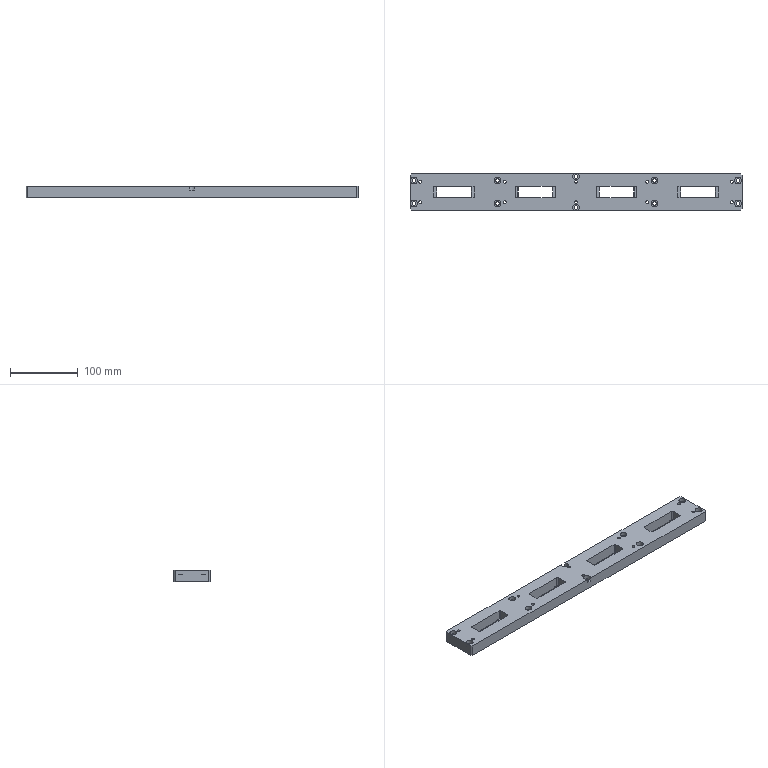NC program | NX | posted with a generic post | part box 490 x 54 x 17 mm
Lines 1 to 1857 of 8955, first 1708 of 1839 lines:
N10 G17 G21 G94 G90
(FLOOR_WALL , TOOL : D80)
N12 T19 M6
N14 G54
N16 G17 G0 G90 X-45. Y-27. S6500 M3
N18 G43 Z30. H19
N20 Z3.
N22 G94 G1 Z0. F1500.
N24 X-42.
N26 X532.
N28 X535.
N30 Z3.
N32 G0 Z30.
N34 M5
(DRILLING , TOOL : D6A45)
N36 T01 M6
N38 G54
N40 G17 G0 G90 X484. Y-10. S5000 M3
N42 G43 Z30. H1
N44 G94 G81 G98 Z-1.8 F350. R3.
N46 X475. Y-12.
N48 X484. Y-44.
N50 X475. Y-42.
N52 X361. Y-44.
N54 X350. Y-42.
N56 X361. Y-10.
N58 X350. Y-12.
N60 X245. Y-4.
N62 Y-12.
N64 Y-42.
N66 Y-50.
N68 X140. Y-42.
N70 X129. Y-44.
N72 X140. Y-12.
N74 X129. Y-10.
N76 X15. Y-12.
N78 X6. Y-10.
N80 X15. Y-42.
N82 X6. Y-44.
N84 G80
N86 G0 X6. Y-44. Z30.
N88 M5
(DRILLING_COPY_COPY , TOOL : 4..2ZT)
N90 T04 M6
N92 G54
N94 G17 G0 G90 X15. Y-12. S2000 M3
N96 G43 Z30. H4
N98 G94 G83 G98 Z-19.762 F300. Q2. R3.
N100 Y-42.
N102 X140.
N104 Y-12.
N106 X245.
N108 Y-42.
N110 X350.
N112 Y-12.
N114 X475.
N116 Y-42.
N118 G80
N120 G0 X475. Y-42. Z30.
N122 M5
(DRILLING_COPY_COPY_COPY , TOOL : 5.5ZT)
N124 T09 M6
N126 G54
N128 G17 G0 G90 X6. Y-10. S2000 M3
N130 G43 Z30. H9
N132 G94 G83 G98 Z-19.152 F300. Q2. R3.
N134 Y-44.
N136 X129.
N138 Y-10.
N140 X245. Y-4.
N142 Y-50.
N144 X361. Y-44.
N146 Y-10.
N148 X484.
N150 Y-44.
N152 G80
N154 G0 X484. Y-44. Z30.
N156 M5
(ZLEVEL_PROFILE , TOOL : D10)
N158 T15 M6
N160 G54
N162 G17 G0 G90 X423.853 Y-23.5 S8500 M3
N164 G43 Z30. H15
N166 Z1.5
N168 G94 G1 X400.1 Z0.255 F1000.
N170 Y-30.5 Z-0.112
N172 X425. Z-1.417
N174 X449.9 F3000.
N176 Y-23.5
N178 X400.1
N180 Y-30.5
N182 X425.
N184 X449.9 Z-1.727
N186 Y-23.5 Z-1.814
N188 X410.06 Z-2.311
N190 X405.08 Z-2.373
N192 X400.1 Z-2.436
N194 Y-30.5 Z-2.523
N196 X425. Z-2.833
N198 X449.9 Z-3.144
N200 Y-23.5 Z-3.231
N202 X410.06 Z-3.728
N204 X405.08 Z-3.79
N206 X400.1 Z-3.852
N208 Y-30.5 Z-3.939
N210 X425. Z-4.25
N212 X449.9 Z-4.561
N214 Y-23.5 Z-4.648
N216 X410.06 Z-5.145
N218 X405.08 Z-5.207
N220 X400.1 Z-5.269
N222 Y-30.5 Z-5.356
N224 X425. Z-5.667
N226 X449.9 Z-5.977
N228 Y-23.5 Z-6.064
N230 X410.06 Z-6.561
N232 X405.08 Z-6.623
N234 X400.1 Z-6.686
N236 Y-30.5 Z-6.773
N238 X425. Z-7.083
N240 X449.9 Z-7.394
N242 Y-23.5 Z-7.481
N244 X410.06 Z-7.978
N246 X405.08 Z-8.04
N248 X400.1 Y-23.501 Z-8.102
N250 Y-30.5 Z-8.189
N252 X425. Z-8.5
N254 X449.9 Z-8.811
N256 Y-23.5 Z-8.898
N258 X410.061 Z-9.395
N260 X405.08 Z-9.457
N262 X400.1 Y-23.501 Z-9.519
N264 Y-30.5 Z-9.606
N266 X425. Z-9.917
N268 X449.9 Z-10.227
N270 Y-23.5 Z-10.314
N272 X410.061 Z-10.811
N274 X405.08 Z-10.873
N276 X400.1 Y-23.501 Z-10.936
N278 Y-30.5 Z-11.023
N280 X425. Z-11.333
N282 X449.9 Z-11.644
N284 Y-23.5 Z-11.731
N286 X410.061 Z-12.228
N288 X405.08 Z-12.29
N290 X400.1 Y-23.501 Z-12.352
N292 Y-30.5 Z-12.439
N294 X425. Z-12.75
N296 X449.9 Z-13.061
N298 Y-23.5 Z-13.148
N300 X410.061 Z-13.645
N302 X405.08 Z-13.707
N304 X400.1 Y-23.501 Z-13.769
N306 Y-30.5 Z-13.856
N308 X425. Z-14.167
N310 X441.6 Z-14.391
N312 X443.734 Z-14.441
N314 X445.868 Z-14.491
N316 X445.866 Y-30.366 Z-14.492
N318 X445.773 Y-23.503 Z-14.585
N320 X442.858 Y-23.5 Z-14.644
N322 X439.94 Z-14.703
N324 X410.061 Z-15.108
N326 X407.33 Z-15.153
N328 X404.6 Y-23.501 Z-15.199
N330 Y-30.345 Z-15.292
N332 Y-30.5
N334 X408.4 Z-15.294
N336 X416.7 Z-15.359
N338 X425. Z-15.471
N340 Z-15.583
N342 X438.602 Z-15.785
N344 X442.003 Z-15.835
N346 X445.4 Y-30.497 Z-15.886
N348 Y-30.369 Z-15.888
N350 Y-23.5 Z-15.989
N352 X404.6 Z-16.594
N354 Y-30.497 Z-16.698
N356 X407.998 Y-30.5 Z-16.748
N358 X411.399 Z-16.798
N360 X425. Z-17.
N362 X445.403
N364 X445.4 Y-30.366
N366 Y-23.5
N368 X404.6
N370 Y-30.5
N372 X425.
N374 Z-15.5
N376 G0 Z30.
N378 X303.853 Y-23.5
N380 Z1.5
N382 G1 X280.1 Z0.255 F1000.
N384 Y-30.5 Z-0.112
N386 X305. Z-1.417
N388 X329.9 F3000.
N390 Y-23.5
N392 X280.1
N394 Y-30.5
N396 X305.
N398 X329.9 Z-1.727
N400 Y-23.5 Z-1.814
N402 X290.06 Z-2.311
N404 X285.08 Z-2.373
N406 X280.1 Z-2.436
N408 Y-30.5 Z-2.523
N410 X305. Z-2.833
N412 X329.9 Z-3.144
N414 Y-23.5 Z-3.231
N416 X290.06 Z-3.728
N418 X285.08 Z-3.79
N420 X280.1 Z-3.852
N422 Y-30.5 Z-3.939
N424 X305. Z-4.25
N426 X329.9 Z-4.561
N428 Y-23.5 Z-4.648
N430 X290.06 Z-5.145
N432 X285.08 Z-5.207
N434 X280.1 Z-5.269
N436 Y-30.5 Z-5.356
N438 X305. Z-5.667
N440 X329.9 Z-5.977
N442 Y-23.5 Z-6.064
N444 X290.06 Z-6.561
N446 X285.08 Z-6.623
N448 X280.1 Z-6.686
N450 Y-30.5 Z-6.773
N452 X305. Z-7.083
N454 X329.9 Z-7.394
N456 Y-23.5 Z-7.481
N458 X290.06 Z-7.978
N460 X285.08 Z-8.04
N462 X280.1 Y-23.501 Z-8.102
N464 Y-30.5 Z-8.189
N466 X305. Z-8.5
N468 X329.9 Z-8.811
N470 Y-23.5 Z-8.898
N472 X290.061 Z-9.395
N474 X285.08 Z-9.457
N476 X280.1 Y-23.501 Z-9.519
N478 Y-30.5 Z-9.606
N480 X305. Z-9.917
N482 X329.9 Z-10.227
N484 Y-23.5 Z-10.314
N486 X290.061 Z-10.811
N488 X285.08 Z-10.873
N490 X280.1 Y-23.501 Z-10.936
N492 Y-30.5 Z-11.023
N494 X305. Z-11.333
N496 X329.9 Z-11.644
N498 Y-23.5 Z-11.731
N500 X290.061 Z-12.228
N502 X285.08 Z-12.29
N504 X280.1 Y-23.501 Z-12.352
N506 Y-30.5 Z-12.439
N508 X305. Z-12.75
N510 X329.9 Z-13.061
N512 Y-23.5 Z-13.148
N514 X290.061 Z-13.645
N516 X285.08 Z-13.707
N518 X280.1 Y-23.501 Z-13.769
N520 Y-30.5 Z-13.856
N522 X305. Z-14.167
N524 X321.6 Z-14.391
N526 X323.734 Z-14.441
N528 X325.868 Z-14.491
N530 X325.867 Y-30.389 Z-14.492
N532 X325.773 Y-23.503 Z-14.585
N534 X322.858 Y-23.5 Z-14.644
N536 X319.94 Z-14.703
N538 X290.061 Z-15.108
N540 X287.33 Z-15.153
N542 X284.6 Y-23.501 Z-15.199
N544 Y-30.497 Z-15.294
N546 X286.499 Y-30.5 Z-15.326
N548 X288.4 Z-15.359
N550 X305. Z-15.583
N552 X318.602 Z-15.785
N554 X322.002 Z-15.835
N556 X325.4 Y-30.497 Z-15.886
N558 Y-30.389 Z-15.887
N560 Y-23.5 Z-15.989
N562 X284.6 Z-16.594
N564 Y-30.5 Z-16.698
N566 X305. Z-17.
N568 X325.402
N570 X325.4 Y-30.389
N572 Y-23.5
N574 X284.6
N576 Y-30.5
N578 X305.
N580 Z-15.5
N582 G0 Z30.
N584 X183.853 Y-23.5
N586 Z1.5
N588 G1 X160.1 Z0.255 F1000.
N590 Y-30.5 Z-0.112
N592 X185. Z-1.417
N594 X209.9 F3000.
N596 Y-23.5
N598 X160.1
N600 Y-30.5
N602 X185.
N604 X209.9 Z-1.727
N606 Y-23.5 Z-1.814
N608 X160.1 Z-2.436
N610 Y-30.5 Z-2.523
N612 X185. Z-2.833
N614 X209.9 Z-3.144
N616 Y-23.5 Z-3.231
N618 X160.1 Z-3.852
N620 Y-30.5 Z-3.939
N622 X185. Z-4.25
N624 X209.9 Z-4.561
N626 Y-23.5 Z-4.648
N628 X160.1 Z-5.269
N630 Y-30.5 Z-5.356
N632 X185. Z-5.667
N634 X209.9 Z-5.977
N636 Y-23.5 Z-6.064
N638 X160.1 Z-6.686
N640 Y-30.5 Z-6.773
N642 X185. Z-7.083
N644 X209.9 Z-7.394
N646 Y-23.5 Z-7.481
N648 X160.1 Z-8.102
N650 Y-30.5 Z-8.189
N652 X185. Z-8.5
N654 X209.9 Z-8.811
N656 Y-23.5 Z-8.898
N658 X160.1 Z-9.519
N660 Y-30.5 Z-9.606
N662 X185. Z-9.917
N664 X209.9 Z-10.227
N666 Y-23.5 Z-10.314
N668 X160.1 Z-10.936
N670 Y-30.5 Z-11.023
N672 X185. Z-11.333
N674 X209.9 Z-11.644
N676 Y-23.5 Z-11.731
N678 X160.1 Z-12.352
N680 Y-30.5 Z-12.439
N682 X185. Z-12.75
N684 X209.9 Z-13.061
N686 Y-23.5 Z-13.148
N688 X160.1 Z-13.769
N690 Y-30.5 Z-13.856
N692 X185. Z-14.167
N694 X201.6 Z-14.391
N696 X203.736 Z-14.441
N698 X205.868 Y-30.497 Z-14.491
N700 X205.773 Y-23.503 Z-14.585
N702 X202.858 Y-23.5 Z-14.644
N704 X199.94 Z-14.703
N706 X170.06 Z-15.108
N708 X167.329 Z-15.153
N710 X164.6 Y-23.503 Z-15.199
N712 Y-30.497 Z-15.294
N714 X166.499 Y-30.5 Z-15.326
N716 X168.4 Z-15.359
N718 X185. Z-15.583
N720 X205.4 Z-15.886
N722 Y-23.5 Z-15.989
N724 X164.6 Z-16.594
N726 Y-30.5 Z-16.698
N728 X185. Z-17.
N730 X205.4
N732 Y-23.5
N734 X164.6
N736 Y-30.5
N738 X185.
N740 Z-15.5
N742 G0 Z30.
N744 X63.853 Y-23.5
N746 Z1.5
N748 G1 X40.1 Z0.255 F1000.
N750 Y-30.5 Z-0.112
N752 X65. Z-1.417
N754 X89.9 F3000.
N756 Y-23.5
N758 X40.1
N760 Y-30.5
N762 X65.
N764 X89.9 Z-1.727
N766 Y-23.5 Z-1.814
N768 X84.92 Z-1.877
N770 X79.94 Z-1.939
N772 X50.06 Z-2.311
N774 X45.08 Z-2.373
N776 X40.1 Z-2.436
N778 Y-30.5 Z-2.523
N780 X65. Z-2.833
N782 X89.9 Z-3.144
N784 Y-23.5 Z-3.231
N786 X84.92 Z-3.293
N788 X79.94 Z-3.355
N790 X50.06 Z-3.728
N792 X45.08 Z-3.79
N794 X40.1 Z-3.852
N796 Y-30.5 Z-3.939
N798 X65. Z-4.25
N800 X89.9 Z-4.561
N802 Y-23.5 Z-4.648
N804 X84.92 Z-4.71
N806 X79.94 Z-4.772
N808 X50.06 Z-5.145
N810 X45.08 Z-5.207
N812 X40.1 Z-5.269
N814 Y-30.5 Z-5.356
N816 X65. Z-5.667
N818 X89.9 Z-5.977
N820 Y-23.5 Z-6.064
N822 X84.92 Z-6.127
N824 X79.94 Z-6.189
N826 X50.06 Z-6.561
N828 X45.08 Z-6.623
N830 X40.1 Z-6.686
N832 Y-30.5 Z-6.773
N834 X65. Z-7.083
N836 X89.9 Z-7.394
N838 Y-23.5 Z-7.481
N840 X84.92 Z-7.543
N842 X79.94 Z-7.605
N844 X50.06 Z-7.978
N846 X45.08 Z-8.04
N848 X40.1 Y-23.501 Z-8.102
N850 Y-30.5 Z-8.189
N852 X65. Z-8.5
N854 X89.9 Z-8.811
N856 Y-23.5 Z-8.898
N858 X84.92 Z-8.96
N860 X79.94 Z-9.022
N862 X50.061 Z-9.395
N864 X45.08 Z-9.457
N866 X40.1 Y-23.501 Z-9.519
N868 Y-30.5 Z-9.606
N870 X65. Z-9.917
N872 X89.9 Z-10.227
N874 Y-23.5 Z-10.314
N876 X84.92 Z-10.377
N878 X79.94 Z-10.439
N880 X50.061 Z-10.811
N882 X45.08 Z-10.873
N884 X40.1 Y-23.501 Z-10.936
N886 Y-30.5 Z-11.023
N888 X65. Z-11.333
N890 X89.9 Z-11.644
N892 Y-23.5 Z-11.731
N894 X84.92 Z-11.793
N896 X79.94 Z-11.855
N898 X50.061 Z-12.228
N900 X45.08 Z-12.29
N902 X40.1 Y-23.501 Z-12.352
N904 Y-30.5 Z-12.439
N906 X65. Z-12.75
N908 X89.9 Z-13.061
N910 Y-23.5 Z-13.148
N912 X84.92 Z-13.21
N914 X79.94 Z-13.272
N916 X50.061 Z-13.645
N918 X45.08 Z-13.707
N920 X40.1 Y-23.501 Z-13.769
N922 Y-30.5 Z-13.856
N924 X65. Z-14.167
N926 X81.6 Z-14.391
N928 X83.734 Z-14.441
N930 X85.868 Z-14.491
N932 X85.866 Y-30.345 Z-14.493
N934 X85.773 Y-23.503 Z-14.585
N936 X82.858 Y-23.5 Z-14.644
N938 X79.94 Z-14.703
N940 X50.061 Z-15.108
N942 X47.33 Z-15.153
N944 X44.6 Y-23.501 Z-15.199
N946 Y-30.366 Z-15.292
N948 Y-30.5
N950 X48.4 Z-15.294
N952 X56.7 Z-15.359
N954 X65. Z-15.471
N956 Z-15.583
N958 X78.602 Z-15.785
N960 X82.002 Z-15.835
N962 X85.4 Y-30.497 Z-15.886
N964 Y-30.348 Z-15.888
N966 Y-23.5 Z-15.989
N968 X44.6 Z-16.594
N970 Y-26.934 Z-16.645
N972 Y-30.497 Z-16.698
N974 X47.997 Y-30.5 Z-16.748
N976 X51.398 Z-16.798
N978 X65. Z-17.
N980 X85.402
N982 X85.4 Y-30.345
N984 Y-23.5
N986 X44.6
N988 Y-30.366
N990 X44.597 Y-30.5
N992 X65.
N994 Z-15.5
N996 G0 Z30.
N998 X66.446 Y5.1
N1000 Z1.5
N1002 G1 X122.099 Z-1.417 F1000.
N1004 X242.198 F3000.
N1006 Y5.096
N1008 G2 X245. Y4.124 R5.1
N1010 X247.817 Y5.097 R5.1
N1012 G1 Y5.1
N1014 X488.
N1016 G2 X491.606 Y3.606 R5.1
N1018 G1 X493.606 Y1.606
N1020 G2 X495.1 Y-2. R5.1
N1022 G1 Y-52.
N1024 G2 X493.606 Y-55.606 R5.1
N1026 G1 X491.606 Y-57.606
N1028 G2 X488. Y-59.1 R5.1
N1030 G1 X248.
N1032 G2 X245. Y-58.124 R5.1
N1034 X242. Y-59.1 R5.1
N1036 G1 X2.
N1038 G2 X-1.606 Y-57.606 R5.1
N1040 G1 X-3.606 Y-55.606
N1042 G2 X-5.1 Y-52. R5.1
N1044 G1 Y-2.
N1046 G2 X-3.606 Y1.606 R5.1
N1048 G1 X-1.606 Y3.606
N1050 G2 X2. Y5.1 R5.1
N1052 G1 X122.099
N1054 X232.96 Z-1.557
N1056 X237.58 Z-1.563
N1058 X242.198 Y5.096 Z-1.569
N1060 X242.708 Y5.051 Z-1.57
N1062 X243.19 Y4.959
N1064 X243.671 Y4.818 Z-1.571
N1066 X244.136 Y4.631 Z-1.572
N1068 X244.574 Y4.403
N1070 X245. Y4.124 Z-1.573
N1072 X245.429 Y4.404 Z-1.574
N1074 X245.868 Y4.633
N1076 X246.336 Y4.821 Z-1.575
N1078 X246.82 Y4.962
N1080 X247.305 Y5.052 Z-1.576
N1082 X247.817 Y5.097 Z-1.577
N1084 X252.62 Y5.1 Z-1.583
N1086 X257.425 Z-1.589
N1088 X488. Z-1.882
N1090 X488.5 Y5.075
N1092 X488.995 Y5.002 Z-1.883
N1094 X489.48 Y4.88 Z-1.884
N1096 X489.952 Y4.712
N1098 X490.404 Y4.498 Z-1.885
N1100 X490.833 Y4.24
N1102 X491.235 Y3.942 Z-1.886
N1104 X491.606 Y3.606 Z-1.887
N1106 X493.606 Y1.606 Z-1.89
N1108 X493.942 Y1.235 Z-1.891
N1110 X494.24 Y0.833 Z-1.892
N1112 X494.498 Y0.404
N1114 X494.712 Y-0.048 Z-1.893
N1116 X494.88 Y-0.52
N1118 X495.002 Y-1.005 Z-1.894
N1120 X495.075 Y-1.5 Z-1.895
N1122 X495.1 Y-2.
N1124 Y-52. Z-1.959
N1126 X495.075 Y-52.5
N1128 X495.002 Y-52.995 Z-1.96
N1130 X494.88 Y-53.48 Z-1.961
N1132 X494.712 Y-53.952
N1134 X494.498 Y-54.404 Z-1.962
N1136 X494.24 Y-54.833 Z-1.963
N1138 X493.942 Y-55.235
N1140 X493.606 Y-55.606 Z-1.964
N1142 X491.606 Y-57.606 Z-1.967
N1144 X491.235 Y-57.942 Z-1.968
N1146 X490.833 Y-58.24 Z-1.969
N1148 X490.404 Y-58.498
N1150 X489.952 Y-58.712 Z-1.97
N1152 X489.48 Y-58.88 Z-1.971
N1154 X488.995 Y-59.002
N1156 X488.5 Y-59.075 Z-1.972
N1158 X488. Y-59.1 Z-1.973
N1160 X248. Z-2.277
N1162 X247.466 Y-59.072 Z-2.278
N1164 X246.939 Y-58.988 Z-2.279
N1166 X246.423 Y-58.85
N1168 X245.924 Y-58.658 Z-2.28
N1170 X245.456 Y-58.42 Z-2.281
N1172 X245. Y-58.124
N1174 X244.544 Y-58.42 Z-2.282
N1176 X244.076 Y-58.658 Z-2.283
N1178 X243.577 Y-58.85
N1180 X243.061 Y-58.988 Z-2.284
N1182 X242.534 Y-59.072 Z-2.285
N1184 X242. Y-59.1
N1186 X2. Z-2.59
N1188 X1.5 Y-59.075 Z-2.591
N1190 X1.005 Y-59.002
N1192 X0.52 Y-58.88 Z-2.592
N1194 X0.048 Y-58.712
N1196 X-0.404 Y-58.498 Z-2.593
N1198 X-0.833 Y-58.24 Z-2.594
N1200 X-1.235 Y-57.942
N1202 X-1.606 Y-57.606 Z-2.595
N1204 X-3.606 Y-55.606 Z-2.599
N1206 X-3.942 Y-55.235
N1208 X-4.24 Y-54.833 Z-2.6
N1210 X-4.498 Y-54.404 Z-2.601
N1212 X-4.712 Y-53.952
N1214 X-4.88 Y-53.48 Z-2.602
N1216 X-5.002 Y-52.995
N1218 X-5.075 Y-52.5 Z-2.603
N1220 X-5.1 Y-52. Z-2.604
N1222 Y-2. Z-2.667
N1224 X-5.075 Y-1.5 Z-2.668
N1226 X-5.002 Y-1.005
N1228 X-4.88 Y-0.52 Z-2.669
N1230 X-4.712 Y-0.048 Z-2.67
N1232 X-4.498 Y0.404
N1234 X-4.24 Y0.833 Z-2.671
N1236 X-3.942 Y1.235 Z-2.672
N1238 X-3.606 Y1.606
N1240 X-1.606 Y3.606 Z-2.676
N1242 X-1.235 Y3.942
N1244 X-0.833 Y4.24 Z-2.677
N1246 X-0.404 Y4.498 Z-2.678
N1248 X0.048 Y4.712
N1250 X0.52 Y4.88 Z-2.679
N1252 X1.005 Y5.002 Z-2.68
N1254 X1.5 Y5.075
N1256 X2. Y5.1 Z-2.681
N1258 X122.099 Z-2.833
N1260 X232.96 Z-2.974
N1262 X237.58 Z-2.98
N1264 X242.198 Y5.096 Z-2.986
N1266 X242.708 Y5.051
N1268 X243.19 Y4.959 Z-2.987
N1270 X243.671 Y4.818 Z-2.988
N1272 X244.136 Y4.631
N1274 X244.574 Y4.403 Z-2.989
N1276 X245. Y4.124 Z-2.99
N1278 X245.429 Y4.404
N1280 X245.868 Y4.633 Z-2.991
N1282 X246.336 Y4.821 Z-2.992
N1284 X246.82 Y4.962
N1286 X247.305 Y5.052 Z-2.993
N1288 X247.817 Y5.097
N1290 X252.62 Y5.1 Z-3.
N1292 X257.425 Z-3.006
N1294 X488. Z-3.298
N1296 X488.5 Y5.075 Z-3.299
N1298 X488.995 Y5.002 Z-3.3
N1300 X489.48 Y4.88
N1302 X489.952 Y4.712 Z-3.301
N1304 X490.404 Y4.498
N1306 X490.833 Y4.24 Z-3.302
N1308 X491.235 Y3.942 Z-3.303
N1310 X491.606 Y3.606
N1312 X493.606 Y1.606 Z-3.307
N1314 X493.942 Y1.235 Z-3.308
N1316 X494.24 Y0.833
N1318 X494.498 Y0.404 Z-3.309
N1320 X494.712 Y-0.048
N1322 X494.88 Y-0.52 Z-3.31
N1324 X495.002 Y-1.005 Z-3.311
N1326 X495.075 Y-1.5
N1328 X495.1 Y-2. Z-3.312
N1330 Y-52. Z-3.375
N1332 X495.075 Y-52.5 Z-3.376
N1334 X495.002 Y-52.995 Z-3.377
N1336 X494.88 Y-53.48
N1338 X494.712 Y-53.952 Z-3.378
N1340 X494.498 Y-54.404 Z-3.379
N1342 X494.24 Y-54.833
N1344 X493.942 Y-55.235 Z-3.38
N1346 X493.606 Y-55.606 Z-3.381
N1348 X491.606 Y-57.606 Z-3.384
N1350 X491.235 Y-57.942 Z-3.385
N1352 X490.833 Y-58.24
N1354 X490.404 Y-58.498 Z-3.386
N1356 X489.952 Y-58.712 Z-3.387
N1358 X489.48 Y-58.88
N1360 X488.995 Y-59.002 Z-3.388
N1362 X488.5 Y-59.075 Z-3.389
N1364 X488. Y-59.1
N1366 X248. Z-3.694
N1368 X247.466 Y-59.072 Z-3.695
N1370 X246.939 Y-58.988
N1372 X246.423 Y-58.85 Z-3.696
N1374 X245.924 Y-58.658 Z-3.697
N1376 X245.456 Y-58.42
N1378 X245. Y-58.124 Z-3.698
N1380 X244.544 Y-58.42 Z-3.699
N1382 X244.076 Y-58.658
N1384 X243.577 Y-58.85 Z-3.7
N1386 X243.061 Y-58.988 Z-3.701
N1388 X242.534 Y-59.072
N1390 X242. Y-59.1 Z-3.702
N1392 X2. Z-4.007
N1394 X1.5 Y-59.075
N1396 X1.005 Y-59.002 Z-4.008
N1398 X0.52 Y-58.88 Z-4.009
N1400 X0.048 Y-58.712
N1402 X-0.404 Y-58.498 Z-4.01
N1404 X-0.833 Y-58.24
N1406 X-1.235 Y-57.942 Z-4.011
N1408 X-1.606 Y-57.606 Z-4.012
N1410 X-3.606 Y-55.606 Z-4.015
N1412 X-3.942 Y-55.235 Z-4.016
N1414 X-4.24 Y-54.833 Z-4.017
N1416 X-4.498 Y-54.404
N1418 X-4.712 Y-53.952 Z-4.018
N1420 X-4.88 Y-53.48
N1422 X-5.002 Y-52.995 Z-4.019
N1424 X-5.075 Y-52.5 Z-4.02
N1426 X-5.1 Y-52.
N1428 Y-2. Z-4.084
N1430 X-5.075 Y-1.5
N1432 X-5.002 Y-1.005 Z-4.085
N1434 X-4.88 Y-0.52 Z-4.086
N1436 X-4.712 Y-0.048
N1438 X-4.498 Y0.404 Z-4.087
N1440 X-4.24 Y0.833 Z-4.088
N1442 X-3.942 Y1.235
N1444 X-3.606 Y1.606 Z-4.089
N1446 X-1.606 Y3.606 Z-4.092
N1448 X-1.235 Y3.942 Z-4.093
N1450 X-0.833 Y4.24 Z-4.094
N1452 X-0.404 Y4.498
N1454 X0.048 Y4.712 Z-4.095
N1456 X0.52 Y4.88 Z-4.096
N1458 X1.005 Y5.002
N1460 X1.5 Y5.075 Z-4.097
N1462 X2. Y5.1 Z-4.098
N1464 X122.099 Z-4.25
N1466 X232.96 Z-4.391
N1468 X237.578 Z-4.397
N1470 X242.194 Y5.096 Z-4.402
N1472 X242.34 Y5.089 Z-4.403
N1474 X242.766 Y5.042
N1476 X243.19 Y4.959 Z-4.404
N1478 X243.663 Y4.821
N1480 X244.136 Y4.631 Z-4.405
N1482 X244.568 Y4.406 Z-4.406
N1484 X245. Y4.124
N1486 X245.434 Y4.408 Z-4.407
N1488 X245.868 Y4.633 Z-4.408
N1490 X246.344 Y4.824
N1492 X246.82 Y4.962 Z-4.409
N1494 X247.239 Y5.043
N1496 X247.66 Y5.089 Z-4.41
N1498 X247.821 Y5.097
N1500 X252.622 Y5.1 Z-4.416
N1502 X257.425 Z-4.422
N1504 X488. Z-4.715
N1506 X488.5 Y5.075 Z-4.716
N1508 X488.995 Y5.002
N1510 X489.48 Y4.88 Z-4.717
N1512 X489.952 Y4.712 Z-4.718
N1514 X490.404 Y4.498
N1516 X490.833 Y4.24 Z-4.719
N1518 X491.235 Y3.942
N1520 X491.606 Y3.606 Z-4.72
N1522 X493.606 Y1.606 Z-4.724
N1524 X493.942 Y1.235
N1526 X494.24 Y0.833 Z-4.725
N1528 X494.498 Y0.404 Z-4.726
N1530 X494.712 Y-0.048
N1532 X494.88 Y-0.52 Z-4.727
N1534 X495.002 Y-1.005 Z-4.728
N1536 X495.075 Y-1.5
N1538 X495.1 Y-2. Z-4.729
N1540 Y-52. Z-4.792
N1542 X495.075 Y-52.5 Z-4.793
N1544 X495.002 Y-52.995 Z-4.794
N1546 X494.88 Y-53.48
N1548 X494.712 Y-53.952 Z-4.795
N1550 X494.498 Y-54.404
N1552 X494.24 Y-54.833 Z-4.796
N1554 X493.942 Y-55.235 Z-4.797
N1556 X493.606 Y-55.606
N1558 X491.606 Y-57.606 Z-4.801
N1560 X491.235 Y-57.942 Z-4.802
N1562 X490.833 Y-58.24
N1564 X490.404 Y-58.498 Z-4.803
N1566 X489.952 Y-58.712
N1568 X489.48 Y-58.88 Z-4.804
N1570 X488.995 Y-59.002 Z-4.805
N1572 X488.5 Y-59.075
N1574 X488. Y-59.1 Z-4.806
N1576 X248. Z-5.111
N1578 X247.469 Y-59.072
N1580 X246.939 Y-58.988 Z-5.112
N1582 X246.431 Y-58.853 Z-5.113
N1584 X245.924 Y-58.658
N1586 X245.462 Y-58.424 Z-5.114
N1588 X245. Y-58.124 Z-5.115
N1590 X244.538 Y-58.424
N1592 X244.076 Y-58.658 Z-5.116
N1594 X243.569 Y-58.853
N1596 X243.061 Y-58.988 Z-5.117
N1598 X242.531 Y-59.072 Z-5.118
N1600 X242. Y-59.1
N1602 X2. Z-5.423
N1604 X1.5 Y-59.075 Z-5.424
N1606 X1.005 Y-59.002
N1608 X0.52 Y-58.88 Z-5.425
N1610 X0.048 Y-58.712 Z-5.426
N1612 X-0.404 Y-58.498
N1614 X-0.833 Y-58.24 Z-5.427
N1616 X-1.235 Y-57.942 Z-5.428
N1618 X-1.606 Y-57.606
N1620 X-3.606 Y-55.606 Z-5.432
N1622 X-3.942 Y-55.235
N1624 X-4.24 Y-54.833 Z-5.433
N1626 X-4.498 Y-54.404 Z-5.434
N1628 X-4.712 Y-53.952
N1630 X-4.88 Y-53.48 Z-5.435
N1632 X-5.002 Y-52.995 Z-5.436
N1634 X-5.075 Y-52.5
N1636 X-5.1 Y-52. Z-5.437
N1638 Y-2. Z-5.5
N1640 X-5.075 Y-1.5 Z-5.501
N1642 X-5.002 Y-1.005 Z-5.502
N1644 X-4.88 Y-0.52
N1646 X-4.712 Y-0.048 Z-5.503
N1648 X-4.498 Y0.404 Z-5.504
N1650 X-4.24 Y0.833
N1652 X-3.942 Y1.235 Z-5.505
N1654 X-3.606 Y1.606 Z-5.506
N1656 X-1.606 Y3.606 Z-5.509
N1658 X-1.235 Y3.942 Z-5.51
N1660 X-0.833 Y4.24
N1662 X-0.404 Y4.498 Z-5.511
N1664 X0.048 Y4.712 Z-5.512
N1666 X0.52 Y4.88
N1668 X1.005 Y5.002 Z-5.513
N1670 X1.5 Y5.075 Z-5.514
N1672 X2. Y5.1
N1674 X122.099 Z-5.667
N1676 X242.34 Z-5.819
N1678 X257.425 Z-5.839
N1680 X488. Z-6.131
N1682 X488.5 Y5.075 Z-6.132
N1684 X488.995 Y5.002 Z-6.133
N1686 X489.48 Y4.88
N1688 X489.952 Y4.712 Z-6.134
N1690 X490.404 Y4.498 Z-6.135
N1692 X490.833 Y4.24
N1694 X491.235 Y3.942 Z-6.136
N1696 X491.606 Y3.606 Z-6.137
N1698 X493.606 Y1.606 Z-6.14
N1700 X493.942 Y1.235 Z-6.141
N1702 X494.24 Y0.833
N1704 X494.498 Y0.404 Z-6.142
N1706 X494.712 Y-0.048 Z-6.143
N1708 X494.88 Y-0.52
N1710 X495.002 Y-1.005 Z-6.144
N1712 X495.075 Y-1.5 Z-6.145
N1714 X495.1 Y-2.
N1716 Y-52. Z-6.209
N1718 X495.075 Y-52.5
N1720 X495.002 Y-52.995 Z-6.21
N1722 X494.88 Y-53.48 Z-6.211
N1724 X494.712 Y-53.952
N1726 X494.498 Y-54.404 Z-6.212
N1728 X494.24 Y-54.833 Z-6.213
N1730 X493.942 Y-55.235
N1732 X493.606 Y-55.606 Z-6.214
N1734 X491.606 Y-57.606 Z-6.217
N1736 X491.235 Y-57.942 Z-6.218
N1738 X490.833 Y-58.24 Z-6.219
N1740 X490.404 Y-58.498
N1742 X489.952 Y-58.712 Z-6.22
N1744 X489.48 Y-58.88 Z-6.221
N1746 X488.995 Y-59.002
N1748 X488.5 Y-59.075 Z-6.222
N1750 X488. Y-59.1
N1752 X247.878 Z-6.527
N1754 X232. Z-6.548
N1756 X2. Z-6.84
N1758 X1.5 Y-59.075
N1760 X1.005 Y-59.002 Z-6.841
N1762 X0.52 Y-58.88 Z-6.842
N1764 X0.048 Y-58.712
N1766 X-0.404 Y-58.498 Z-6.843
N1768 X-0.833 Y-58.24 Z-6.844
N1770 X-1.235 Y-57.942
N1772 X-1.606 Y-57.606 Z-6.845
N1774 X-3.606 Y-55.606 Z-6.848
N1776 X-3.942 Y-55.235 Z-6.849
N1778 X-4.24 Y-54.833 Z-6.85
N1780 X-4.498 Y-54.404
N1782 X-4.712 Y-53.952 Z-6.851
N1784 X-4.88 Y-53.48 Z-6.852
N1786 X-5.002 Y-52.995
N1788 X-5.075 Y-52.5 Z-6.853
N1790 X-5.1 Y-52. Z-6.854
N1792 Y-2. Z-6.917
N1794 X-5.075 Y-1.5 Z-6.918
N1796 X-5.002 Y-1.005
N1798 X-4.88 Y-0.52 Z-6.919
N1800 X-4.712 Y-0.048 Z-6.92
N1802 X-4.498 Y0.404
N1804 X-4.24 Y0.833 Z-6.921
N1806 X-3.942 Y1.235
N1808 X-3.606 Y1.606 Z-6.922
N1810 X-1.606 Y3.606 Z-6.926
N1812 X-1.235 Y3.942
N1814 X-0.833 Y4.24 Z-6.927
N1816 X-0.404 Y4.498 Z-6.928
N1818 X0.048 Y4.712
N1820 X0.52 Y4.88 Z-6.929
N1822 X1.005 Y5.002 Z-6.93
N1824 X1.5 Y5.075
N1826 X2. Y5.1 Z-6.931
N1828 X122.099 Z-7.083
N1830 X488. Z-7.548
N1832 X488.5 Y5.075 Z-7.549
N1834 X488.995 Y5.002
N1836 X489.48 Y4.88 Z-7.55
N1838 X489.952 Y4.712 Z-7.551
N1840 X490.404 Y4.498
N1842 X490.833 Y4.24 Z-7.552
N1844 X491.235 Y3.942 Z-7.553
N1846 X491.606 Y3.606
N1848 X493.606 Y1.606 Z-7.557
N1850 X493.942 Y1.235
N1852 X494.24 Y0.833 Z-7.558
N1854 X494.498 Y0.404 Z-7.559
N1856 X494.712 Y-0.048
N1858 X494.88 Y-0.52 Z-7.56
N1860 X495.002 Y-1.005 Z-7.561
N1862 X495.075 Y-1.5
N1864 X495.1 Y-2. Z-7.562
N1866 Y-52. Z-7.625
N1868 X495.075 Y-52.5 Z-7.626
N1870 X495.002 Y-52.995 Z-7.627
N1872 X494.88 Y-53.48
N1874 X494.712 Y-53.952 Z-7.628
N1876 X494.498 Y-54.404 Z-7.629
N1878 X494.24 Y-54.833
N1880 X493.942 Y-55.235 Z-7.63
N1882 X493.606 Y-55.606
N1884 X491.606 Y-57.606 Z-7.634
N1886 X491.235 Y-57.942 Z-7.635
N1888 X490.833 Y-58.24
N1890 X490.404 Y-58.498 Z-7.636
N1892 X489.952 Y-58.712 Z-7.637
N1894 X489.48 Y-58.88
N1896 X488.995 Y-59.002 Z-7.638
N1898 X488.5 Y-59.075
N1900 X488. Y-59.1 Z-7.639
N1902 X2. Z-8.256
N1904 X1.5 Y-59.075 Z-8.257
N1906 X1.005 Y-59.002 Z-8.258
N1908 X0.52 Y-58.88
N1910 X0.048 Y-58.712 Z-8.259
N1912 X-0.404 Y-58.498 Z-8.26
N1914 X-0.833 Y-58.24
N1916 X-1.235 Y-57.942 Z-8.261
N1918 X-1.606 Y-57.606 Z-8.262
N1920 X-3.606 Y-55.606 Z-8.265
N1922 X-3.942 Y-55.235 Z-8.266
N1924 X-4.24 Y-54.833
N1926 X-4.498 Y-54.404 Z-8.267
N1928 X-4.712 Y-53.952 Z-8.268
N1930 X-4.88 Y-53.48
N1932 X-5.002 Y-52.995 Z-8.269
N1934 X-5.075 Y-52.5 Z-8.27
N1936 X-5.1 Y-52.
N1938 Y-2. Z-8.334
N1940 X-5.075 Y-1.5
N1942 X-5.002 Y-1.005 Z-8.335
N1944 X-4.88 Y-0.52 Z-8.336
N1946 X-4.712 Y-0.048
N1948 X-4.498 Y0.404 Z-8.337
N1950 X-4.24 Y0.833 Z-8.338
N1952 X-3.942 Y1.235
N1954 X-3.606 Y1.606 Z-8.339
N1956 X-1.606 Y3.606 Z-8.342
N1958 X-1.235 Y3.942 Z-8.343
N1960 X-0.833 Y4.24 Z-8.344
N1962 X-0.404 Y4.498
N1964 X0.048 Y4.712 Z-8.345
N1966 X0.52 Y4.88 Z-8.346
N1968 X1.005 Y5.002
N1970 X1.5 Y5.075 Z-8.347
N1972 X2. Y5.1
N1974 X122.099 Z-8.5
N1976 X488. Z-8.965
N1978 X488.5 Y5.075
N1980 X488.995 Y5.002 Z-8.966
N1982 X489.48 Y4.88 Z-8.967
N1984 X489.952 Y4.712
N1986 X490.404 Y4.498 Z-8.968
N1988 X490.833 Y4.24 Z-8.969
N1990 X491.235 Y3.942
N1992 X491.606 Y3.606 Z-8.97
N1994 X493.606 Y1.606 Z-8.973
N1996 X493.942 Y1.235 Z-8.974
N1998 X494.24 Y0.833 Z-8.975
N2000 X494.498 Y0.404
N2002 X494.712 Y-0.048 Z-8.976
N2004 X494.88 Y-0.52 Z-8.977
N2006 X495.002 Y-1.005
N2008 X495.075 Y-1.5 Z-8.978
N2010 X495.1 Y-2. Z-8.979
N2012 Y-52. Z-9.042
N2014 X495.075 Y-52.5 Z-9.043
N2016 X495.002 Y-52.995
N2018 X494.88 Y-53.48 Z-9.044
N2020 X494.712 Y-53.952 Z-9.045
N2022 X494.498 Y-54.404
N2024 X494.24 Y-54.833 Z-9.046
N2026 X493.942 Y-55.235
N2028 X493.606 Y-55.606 Z-9.047
N2030 X491.606 Y-57.606 Z-9.051
N2032 X491.235 Y-57.942
N2034 X490.833 Y-58.24 Z-9.052
N2036 X490.404 Y-58.498 Z-9.053
N2038 X489.952 Y-58.712
N2040 X489.48 Y-58.88 Z-9.054
N2042 X488.995 Y-59.002 Z-9.055
N2044 X488.5 Y-59.075
N2046 X488. Y-59.1 Z-9.056
N2048 X2. Z-9.673
N2050 X1.5 Y-59.075 Z-9.674
N2052 X1.005 Y-59.002
N2054 X0.52 Y-58.88 Z-9.675
N2056 X0.048 Y-58.712 Z-9.676
N2058 X-0.404 Y-58.498
N2060 X-0.833 Y-58.24 Z-9.677
N2062 X-1.235 Y-57.942 Z-9.678
N2064 X-1.606 Y-57.606
N2066 X-3.606 Y-55.606 Z-9.682
N2068 X-3.942 Y-55.235
N2070 X-4.24 Y-54.833 Z-9.683
N2072 X-4.498 Y-54.404 Z-9.684
N2074 X-4.712 Y-53.952
N2076 X-4.88 Y-53.48 Z-9.685
N2078 X-5.002 Y-52.995 Z-9.686
N2080 X-5.075 Y-52.5
N2082 X-5.1 Y-52. Z-9.687
N2084 Y-2. Z-9.75
N2086 X-5.075 Y-1.5 Z-9.751
N2088 X-5.002 Y-1.005 Z-9.752
N2090 X-4.88 Y-0.52
N2092 X-4.712 Y-0.048 Z-9.753
N2094 X-4.498 Y0.404 Z-9.754
N2096 X-4.24 Y0.833
N2098 X-3.942 Y1.235 Z-9.755
N2100 X-3.606 Y1.606
N2102 X-1.606 Y3.606 Z-9.759
N2104 X-1.235 Y3.942 Z-9.76
N2106 X-0.833 Y4.24
N2108 X-0.404 Y4.498 Z-9.761
N2110 X0.048 Y4.712 Z-9.762
N2112 X0.52 Y4.88
N2114 X1.005 Y5.002 Z-9.763
N2116 X1.5 Y5.075
N2118 X2. Y5.1 Z-9.764
N2120 X122.099 Z-9.917
N2122 X488. Z-10.381
N2124 X488.5 Y5.075 Z-10.382
N2126 X488.995 Y5.002 Z-10.383
N2128 X489.48 Y4.88
N2130 X489.952 Y4.712 Z-10.384
N2132 X490.404 Y4.498 Z-10.385
N2134 X490.833 Y4.24
N2136 X491.235 Y3.942 Z-10.386
N2138 X491.606 Y3.606 Z-10.387
N2140 X493.606 Y1.606 Z-10.39
N2142 X493.942 Y1.235 Z-10.391
N2144 X494.24 Y0.833
N2146 X494.498 Y0.404 Z-10.392
N2148 X494.712 Y-0.048 Z-10.393
N2150 X494.88 Y-0.52
N2152 X495.002 Y-1.005 Z-10.394
N2154 X495.075 Y-1.5 Z-10.395
N2156 X495.1 Y-2.
N2158 Y-52. Z-10.459
N2160 X495.075 Y-52.5
N2162 X495.002 Y-52.995 Z-10.46
N2164 X494.88 Y-53.48 Z-10.461
N2166 X494.712 Y-53.952
N2168 X494.498 Y-54.404 Z-10.462
N2170 X494.24 Y-54.833 Z-10.463
N2172 X493.942 Y-55.235
N2174 X493.606 Y-55.606 Z-10.464
N2176 X491.606 Y-57.606 Z-10.467
N2178 X491.235 Y-57.942 Z-10.468
N2180 X490.833 Y-58.24 Z-10.469
N2182 X490.404 Y-58.498
N2184 X489.952 Y-58.712 Z-10.47
N2186 X489.48 Y-58.88 Z-10.471
N2188 X488.995 Y-59.002
N2190 X488.5 Y-59.075 Z-10.472
N2192 X488. Y-59.1
N2194 X2. Z-11.09
N2196 X1.5 Y-59.075
N2198 X1.005 Y-59.002 Z-11.091
N2200 X0.52 Y-58.88 Z-11.092
N2202 X0.048 Y-58.712
N2204 X-0.404 Y-58.498 Z-11.093
N2206 X-0.833 Y-58.24 Z-11.094
N2208 X-1.235 Y-57.942
N2210 X-1.606 Y-57.606 Z-11.095
N2212 X-3.606 Y-55.606 Z-11.098
N2214 X-3.942 Y-55.235 Z-11.099
N2216 X-4.24 Y-54.833 Z-11.1
N2218 X-4.498 Y-54.404
N2220 X-4.712 Y-53.952 Z-11.101
N2222 X-4.88 Y-53.48 Z-11.102
N2224 X-5.002 Y-52.995
N2226 X-5.075 Y-52.5 Z-11.103
N2228 X-5.1 Y-52. Z-11.104
N2230 Y-2. Z-11.167
N2232 X-5.075 Y-1.5 Z-11.168
N2234 X-5.002 Y-1.005
N2236 X-4.88 Y-0.52 Z-11.169
N2238 X-4.712 Y-0.048 Z-11.17
N2240 X-4.498 Y0.404
N2242 X-4.24 Y0.833 Z-11.171
N2244 X-3.942 Y1.235
N2246 X-3.606 Y1.606 Z-11.172
N2248 X-1.606 Y3.606 Z-11.176
N2250 X-1.235 Y3.942
N2252 X-0.833 Y4.24 Z-11.177
N2254 X-0.404 Y4.498 Z-11.178
N2256 X0.048 Y4.712
N2258 X0.52 Y4.88 Z-11.179
N2260 X1.005 Y5.002 Z-11.18
N2262 X1.5 Y5.075
N2264 X2. Y5.1 Z-11.181
N2266 X122.099 Z-11.333
N2268 X488. Z-11.798
N2270 X488.5 Y5.075 Z-11.799
N2272 X488.995 Y5.002
N2274 X489.48 Y4.88 Z-11.8
N2276 X489.952 Y4.712 Z-11.801
N2278 X490.404 Y4.498
N2280 X490.833 Y4.24 Z-11.802
N2282 X491.235 Y3.942 Z-11.803
N2284 X491.606 Y3.606
N2286 X493.606 Y1.606 Z-11.807
N2288 X493.942 Y1.235
N2290 X494.24 Y0.833 Z-11.808
N2292 X494.498 Y0.404 Z-11.809
N2294 X494.712 Y-0.048
N2296 X494.88 Y-0.52 Z-11.81
N2298 X495.002 Y-1.005 Z-11.811
N2300 X495.075 Y-1.5
N2302 X495.1 Y-2. Z-11.812
N2304 Y-52. Z-11.875
N2306 X495.075 Y-52.5 Z-11.876
N2308 X495.002 Y-52.995 Z-11.877
N2310 X494.88 Y-53.48
N2312 X494.712 Y-53.952 Z-11.878
N2314 X494.498 Y-54.404 Z-11.879
N2316 X494.24 Y-54.833
N2318 X493.942 Y-55.235 Z-11.88
N2320 X493.606 Y-55.606
N2322 X491.606 Y-57.606 Z-11.884
N2324 X491.235 Y-57.942 Z-11.885
N2326 X490.833 Y-58.24
N2328 X490.404 Y-58.498 Z-11.886
N2330 X489.952 Y-58.712 Z-11.887
N2332 X489.48 Y-58.88
N2334 X488.995 Y-59.002 Z-11.888
N2336 X488.5 Y-59.075
N2338 X488. Y-59.1 Z-11.889
N2340 X2. Z-12.506
N2342 X1.5 Y-59.075 Z-12.507
N2344 X1.005 Y-59.002 Z-12.508
N2346 X0.52 Y-58.88
N2348 X0.048 Y-58.712 Z-12.509
N2350 X-0.404 Y-58.498 Z-12.51
N2352 X-0.833 Y-58.24
N2354 X-1.235 Y-57.942 Z-12.511
N2356 X-1.606 Y-57.606 Z-12.512
N2358 X-3.606 Y-55.606 Z-12.515
N2360 X-3.942 Y-55.235 Z-12.516
N2362 X-4.24 Y-54.833
N2364 X-4.498 Y-54.404 Z-12.517
N2366 X-4.712 Y-53.952 Z-12.518
N2368 X-4.88 Y-53.48
N2370 X-5.002 Y-52.995 Z-12.519
N2372 X-5.075 Y-52.5 Z-12.52
N2374 X-5.1 Y-52.
N2376 Y-2. Z-12.584
N2378 X-5.075 Y-1.5
N2380 X-5.002 Y-1.005 Z-12.585
N2382 X-4.88 Y-0.52 Z-12.586
N2384 X-4.712 Y-0.048
N2386 X-4.498 Y0.404 Z-12.587
N2388 X-4.24 Y0.833 Z-12.588
N2390 X-3.942 Y1.235
N2392 X-3.606 Y1.606 Z-12.589
N2394 X-1.606 Y3.606 Z-12.592
N2396 X-1.235 Y3.942 Z-12.593
N2398 X-0.833 Y4.24 Z-12.594
N2400 X-0.404 Y4.498
N2402 X0.048 Y4.712 Z-12.595
N2404 X0.52 Y4.88 Z-12.596
N2406 X1.005 Y5.002
N2408 X1.5 Y5.075 Z-12.597
N2410 X2. Y5.1
N2412 X122.099 Z-12.75
N2414 X488. Z-13.215
N2416 X488.5 Y5.075
N2418 X488.995 Y5.002 Z-13.216
N2420 X489.48 Y4.88 Z-13.217
N2422 X489.952 Y4.712
N2424 X490.404 Y4.498 Z-13.218
N2426 X490.833 Y4.24 Z-13.219
N2428 X491.235 Y3.942
N2430 X491.606 Y3.606 Z-13.22
N2432 X493.606 Y1.606 Z-13.223
N2434 X493.942 Y1.235 Z-13.224
N2436 X494.24 Y0.833 Z-13.225
N2438 X494.498 Y0.404
N2440 X494.712 Y-0.048 Z-13.226
N2442 X494.88 Y-0.52 Z-13.227
N2444 X495.002 Y-1.005
N2446 X495.075 Y-1.5 Z-13.228
N2448 X495.1 Y-2. Z-13.229
N2450 Y-52. Z-13.292
N2452 X495.075 Y-52.5 Z-13.293
N2454 X495.002 Y-52.995
N2456 X494.88 Y-53.48 Z-13.294
N2458 X494.712 Y-53.952 Z-13.295
N2460 X494.498 Y-54.404
N2462 X494.24 Y-54.833 Z-13.296
N2464 X493.942 Y-55.235
N2466 X493.606 Y-55.606 Z-13.297
N2468 X491.606 Y-57.606 Z-13.301
N2470 X491.235 Y-57.942
N2472 X490.833 Y-58.24 Z-13.302
N2474 X490.404 Y-58.498 Z-13.303
N2476 X489.952 Y-58.712
N2478 X489.48 Y-58.88 Z-13.304
N2480 X488.995 Y-59.002 Z-13.305
N2482 X488.5 Y-59.075
N2484 X488. Y-59.1 Z-13.306
N2486 X2. Z-13.923
N2488 X1.5 Y-59.075 Z-13.924
N2490 X1.005 Y-59.002
N2492 X0.52 Y-58.88 Z-13.925
N2494 X0.048 Y-58.712 Z-13.926
N2496 X-0.404 Y-58.498
N2498 X-0.833 Y-58.24 Z-13.927
N2500 X-1.235 Y-57.942 Z-13.928
N2502 X-1.606 Y-57.606
N2504 X-3.606 Y-55.606 Z-13.932
N2506 X-3.942 Y-55.235
N2508 X-4.24 Y-54.833 Z-13.933
N2510 X-4.498 Y-54.404 Z-13.934
N2512 X-4.712 Y-53.952
N2514 X-4.88 Y-53.48 Z-13.935
N2516 X-5.002 Y-52.995 Z-13.936
N2518 X-5.075 Y-52.5
N2520 X-5.1 Y-52. Z-13.937
N2522 Y-2. Z-14.
N2524 X-5.075 Y-1.5 Z-14.001
N2526 X-5.002 Y-1.005 Z-14.002
N2528 X-4.88 Y-0.52
N2530 X-4.712 Y-0.048 Z-14.003
N2532 X-4.498 Y0.404 Z-14.004
N2534 X-4.24 Y0.833
N2536 X-3.942 Y1.235 Z-14.005
N2538 X-3.606 Y1.606
N2540 X-1.606 Y3.606 Z-14.009
N2542 X-1.235 Y3.942 Z-14.01
N2544 X-0.833 Y4.24
N2546 X-0.404 Y4.498 Z-14.011
N2548 X0.048 Y4.712 Z-14.012
N2550 X0.52 Y4.88
N2552 X1.005 Y5.002 Z-14.013
N2554 X1.5 Y5.075
N2556 X2. Y5.1 Z-14.014
N2558 X122.099 Z-14.167
N2560 X488. Z-14.631
N2562 X488.5 Y5.075 Z-14.632
N2564 X488.995 Y5.002 Z-14.633
N2566 X489.48 Y4.88
N2568 X489.952 Y4.712 Z-14.634
N2570 X490.404 Y4.498 Z-14.635
N2572 X490.833 Y4.24
N2574 X491.235 Y3.942 Z-14.636
N2576 X491.606 Y3.606 Z-14.637
N2578 X493.606 Y1.606 Z-14.64
N2580 X493.942 Y1.235 Z-14.641
N2582 X494.24 Y0.833
N2584 X494.498 Y0.404 Z-14.642
N2586 X494.712 Y-0.048 Z-14.643
N2588 X494.88 Y-0.52
N2590 X495.002 Y-1.005 Z-14.644
N2592 X495.075 Y-1.5 Z-14.645
N2594 X495.1 Y-2.
N2596 Y-52. Z-14.709
N2598 X495.075 Y-52.5
N2600 X495.002 Y-52.995 Z-14.71
N2602 X494.88 Y-53.48 Z-14.711
N2604 X494.712 Y-53.952
N2606 X494.498 Y-54.404 Z-14.712
N2608 X494.24 Y-54.833 Z-14.713
N2610 X493.942 Y-55.235
N2612 X493.606 Y-55.606 Z-14.714
N2614 X491.606 Y-57.606 Z-14.717
N2616 X491.235 Y-57.942 Z-14.718
N2618 X490.833 Y-58.24 Z-14.719
N2620 X490.404 Y-58.498
N2622 X489.952 Y-58.712 Z-14.72
N2624 X489.48 Y-58.88 Z-14.721
N2626 X488.995 Y-59.002
N2628 X488.5 Y-59.075 Z-14.722
N2630 X488. Y-59.1
N2632 X2. Z-15.34
N2634 X1.5 Y-59.075
N2636 X1.005 Y-59.002 Z-15.341
N2638 X0.52 Y-58.88 Z-15.342
N2640 X0.048 Y-58.712
N2642 X-0.404 Y-58.498 Z-15.343
N2644 X-0.833 Y-58.24 Z-15.344
N2646 X-1.235 Y-57.942
N2648 X-1.606 Y-57.606 Z-15.345
N2650 X-3.606 Y-55.606 Z-15.348
N2652 X-3.942 Y-55.235 Z-15.349
N2654 X-4.24 Y-54.833 Z-15.35
N2656 X-4.498 Y-54.404
N2658 X-4.712 Y-53.952 Z-15.351
N2660 X-4.88 Y-53.48 Z-15.352
N2662 X-5.002 Y-52.995
N2664 X-5.075 Y-52.5 Z-15.353
N2666 X-5.1 Y-52. Z-15.354
N2668 Y-2. Z-15.417
N2670 X-5.075 Y-1.5 Z-15.418
N2672 X-5.002 Y-1.005
N2674 X-4.88 Y-0.52 Z-15.419
N2676 X-4.712 Y-0.048 Z-15.42
N2678 X-4.498 Y0.404
N2680 X-4.24 Y0.833 Z-15.421
N2682 X-3.942 Y1.235
N2684 X-3.606 Y1.606 Z-15.422
N2686 X-1.606 Y3.606 Z-15.426
N2688 X-1.235 Y3.942
N2690 X-0.833 Y4.24 Z-15.427
N2692 X-0.404 Y4.498 Z-15.428
N2694 X0.048 Y4.712
N2696 X0.52 Y4.88 Z-15.429
N2698 X1.005 Y5.002 Z-15.43
N2700 X1.5 Y5.075
N2702 X2. Y5.1 Z-15.431
N2704 X122.099 Z-15.583
N2706 X488. Z-16.048
N2708 X488.5 Y5.075 Z-16.049
N2710 X488.995 Y5.002
N2712 X489.48 Y4.88 Z-16.05
N2714 X489.952 Y4.712 Z-16.051
N2716 X490.404 Y4.498
N2718 X490.833 Y4.24 Z-16.052
N2720 X491.235 Y3.942 Z-16.053
N2722 X491.606 Y3.606
N2724 X493.606 Y1.606 Z-16.057
N2726 X493.942 Y1.235
N2728 X494.24 Y0.833 Z-16.058
N2730 X494.498 Y0.404 Z-16.059
N2732 X494.712 Y-0.048
N2734 X494.88 Y-0.52 Z-16.06
N2736 X495.002 Y-1.005 Z-16.061
N2738 X495.075 Y-1.5
N2740 X495.1 Y-2. Z-16.062
N2742 Y-52. Z-16.125
N2744 X495.075 Y-52.5 Z-16.126
N2746 X495.002 Y-52.995 Z-16.127
N2748 X494.88 Y-53.48
N2750 X494.712 Y-53.952 Z-16.128
N2752 X494.498 Y-54.404 Z-16.129
N2754 X494.24 Y-54.833
N2756 X493.942 Y-55.235 Z-16.13
N2758 X493.606 Y-55.606
N2760 X491.606 Y-57.606 Z-16.134
N2762 X491.235 Y-57.942 Z-16.135
N2764 X490.833 Y-58.24
N2766 X490.404 Y-58.498 Z-16.136
N2768 X489.952 Y-58.712 Z-16.137
N2770 X489.48 Y-58.88
N2772 X488.995 Y-59.002 Z-16.138
N2774 X488.5 Y-59.075
N2776 X488. Y-59.1 Z-16.139
N2778 X2. Z-16.756
N2780 X1.5 Y-59.075 Z-16.757
N2782 X1.005 Y-59.002 Z-16.758
N2784 X0.52 Y-58.88
N2786 X0.048 Y-58.712 Z-16.759
N2788 X-0.404 Y-58.498 Z-16.76
N2790 X-0.833 Y-58.24
N2792 X-1.235 Y-57.942 Z-16.761
N2794 X-1.606 Y-57.606 Z-16.762
N2796 X-3.606 Y-55.606 Z-16.765
N2798 X-3.942 Y-55.235 Z-16.766
N2800 X-4.24 Y-54.833
N2802 X-4.498 Y-54.404 Z-16.767
N2804 X-4.712 Y-53.952 Z-16.768
N2806 X-4.88 Y-53.48
N2808 X-5.002 Y-52.995 Z-16.769
N2810 X-5.075 Y-52.5 Z-16.77
N2812 X-5.1 Y-52.
N2814 Y-2. Z-16.834
N2816 X-5.075 Y-1.5
N2818 X-5.002 Y-1.005 Z-16.835
N2820 X-4.88 Y-0.52 Z-16.836
N2822 X-4.712 Y-0.048
N2824 X-4.498 Y0.404 Z-16.837
N2826 X-4.24 Y0.833 Z-16.838
N2828 X-3.942 Y1.235
N2830 X-3.606 Y1.606 Z-16.839
N2832 X-1.606 Y3.606 Z-16.842
N2834 X-1.235 Y3.942 Z-16.843
N2836 X-0.833 Y4.24 Z-16.844
N2838 X-0.404 Y4.498
N2840 X0.048 Y4.712 Z-16.845
N2842 X0.52 Y4.88 Z-16.846
N2844 X1.005 Y5.002
N2846 X1.5 Y5.075 Z-16.847
N2848 X2. Y5.1
N2850 X122.099 Z-17.
N2852 X488.
N2854 G2 X491.606 Y3.606 R5.1
N2856 G1 X493.606 Y1.606
N2858 G2 X495.1 Y-2. R5.1
N2860 G1 Y-52.
N2862 G2 X493.606 Y-55.606 R5.1
N2864 G1 X491.606 Y-57.606
N2866 G2 X488. Y-59.1 R5.1
N2868 G1 X2.
N2870 G2 X-1.606 Y-57.606 R5.1
N2872 G1 X-3.606 Y-55.606
N2874 G2 X-5.1 Y-52. R5.1
N2876 G1 Y-2.
N2878 G2 X-3.606 Y1.606 R5.1
N2880 G1 X-1.606 Y3.606
N2882 G2 X2. Y5.1 R5.1
N2884 G1 X122.099
N2886 Z-15.5
N2888 G0 Z30.
N2890 M5
(ZLEVEL_PROFILE_1 , TOOL : D10JING)
N2892 T14 M6
N2894 G54
N2896 G17 G0 G90 X46.964 Y-28.6 S8500 M3
N2898 G43 Z30. H14
N2900 Z-15.5
N2902 G94 G1 Z-17. F1000.
N2904 X45. Y-29.734
N2906 G3 X44.5 Y-30.6 R1.
N2908 G1 X85.5 F1500.
N2910 Y-23.4
N2912 X44.5
N2914 Y-30.6
N2916 G3 X45.366 Y-30.1 R1.
N2918 G1 X46.5 Y-28.136
N2920 Z-15.5
N2922 G0 Z53.
N2924 X166.964 Y-28.6
N2926 Z-15.5
N2928 G1 Z-17. F1000.
N2930 X165. Y-29.734
N2932 G3 X164.5 Y-30.6 R1.
N2934 G1 X205.5 F1500.
N2936 Y-23.4
N2938 X164.5
N2940 Y-30.6
N2942 G3 X165.366 Y-30.1 R1.
N2944 G1 X166.5 Y-28.136
N2946 Z-15.5
N2948 G0 Z53.
N2950 X406.964 Y-28.6
N2952 Z-15.5
N2954 G1 Z-17. F1000.
N2956 X405. Y-29.734
N2958 G3 X404.5 Y-30.6 R1.
N2960 G1 X445.5 F1500.
N2962 Y-23.4
N2964 X404.5
N2966 Y-30.6
N2968 G3 X405.366 Y-30.1 R1.
N2970 G1 X406.5 Y-28.136
N2972 Z-15.5
N2974 G0 Z53.
N2976 X286.964 Y-28.6
N2978 Z-15.5
N2980 G1 Z-17. F1000.
N2982 X285. Y-29.734
N2984 G3 X284.5 Y-30.6 R1.
N2986 G1 X325.5 F1500.
N2988 Y-23.4
N2990 X284.5
N2992 Y-30.6
N2994 G3 X285.366 Y-30.1 R1.
N2996 G1 X286.5 Y-28.136
N2998 Z-15.5
N3000 G0 Z53.
N3002 X489.622 Y-60.809
N3004 Z-15.5
N3006 G1 Z-17. F1000.
N3008 X488.866 Y-59.5
N3010 G3 X488. Y-59. R1.
N3012 G1 X2. F1500.
N3014 G2 X-1.536 Y-57.536 R5.
N3016 G1 X-3.536 Y-55.536
N3018 G2 X-5. Y-52. R5.
N3020 G1 Y-2.
N3022 G2 X-3.536 Y1.536 R5.
N3024 G1 X-1.536 Y3.536
N3026 G2 X2. Y5. R5.
N3028 G1 X488.
N3030 G2 X491.536 Y3.536 R5.
N3032 G1 X493.536 Y1.536
N3034 G2 X495. Y-2. R5.
N3036 G1 Y-52.
N3038 G2 X493.536 Y-55.536 R5.
N3040 G1 X491.536 Y-57.536
N3042 G2 X488. Y-59. R5.
N3044 G3 X487.134 Y-59.5 R1.
N3046 G1 X486.268 Y-61.
N3048 Z-15.5
N3050 G0 Z30.
(ZLEVEL_PROFILE_1_COPY , TOOL : D10JING)
N3052 X327.536 Y-25.4
N3054 Z-13.
N3056 G1 Z-14.5 F1000.
N3058 X329.5 Y-24.266
N3060 G3 X330. Y-23.4 R1.
N3062 G1 X280. F1500.
N3064 Y-30.599
N3066 X280.001 Y-30.6
N3068 X330.
N3070 Y-23.4
N3072 G3 X329.134 Y-23.9 R1.
N3074 G1 X328. Y-25.864
N3076 Z-13.
N3078 G0 Z30.
N3080 X323.036 Y-25.4
N3082 Z-15.5
N3084 G1 Z-17. F1000.
N3086 X325. Y-24.266
N3088 G3 X325.5 Y-23.4 R1.
N3090 G1 X284.5 F1500.
N3092 Y-30.6
N3094 X325.5
N3096 Y-23.4
N3098 G3 X324.634 Y-23.9 R1.
N3100 G1 X323.5 Y-25.864
N3102 Z-15.5
N3104 G0 Z30.
N3106 X402.464 Y-28.6
N3108 Z-13.
N3110 G1 Z-14.5 F1000.
N3112 X400.5 Y-29.734
N3114 G3 X400. Y-30.6 R1.
N3116 G1 X450. F1500.
N3118 Y-23.4
N3120 X400.
N3122 Y-30.6
N3124 G3 X400.866 Y-30.1 R1.
N3126 G1 X402. Y-28.136
N3128 Z-13.
N3130 G0 Z30.
N3132 X406.964 Y-28.6
N3134 Z-15.5
N3136 G1 Z-17. F1000.
N3138 X405. Y-29.734
N3140 G3 X404.5 Y-30.6 R1.
N3142 G1 X445.5 F1500.
N3144 Y-23.4
N3146 X404.5
N3148 Y-30.6
N3150 G3 X405.366 Y-30.1 R1.
N3152 G1 X406.5 Y-28.136
N3154 Z-15.5
N3156 G0 Z30.
N3158 X162.464 Y-28.6
N3160 Z-13.
N3162 G1 Z-14.5 F1000.
N3164 X160.5 Y-29.734
N3166 G3 X160. Y-30.6 R1.
N3168 G1 X210. F1500.
N3170 Y-23.4
N3172 X160.
N3174 Y-30.6
N3176 G3 X160.866 Y-30.1 R1.
N3178 G1 X162. Y-28.136
N3180 Z-13.
N3182 G0 Z30.
N3184 X166.964 Y-28.6
N3186 Z-15.5
N3188 G1 Z-17. F1000.
N3190 X165. Y-29.734
N3192 G3 X164.5 Y-30.6 R1.
N3194 G1 X205.5 F1500.
N3196 Y-23.4
N3198 X164.5
N3200 Y-30.6
N3202 G3 X165.366 Y-30.1 R1.
N3204 G1 X166.5 Y-28.136
N3206 Z-15.5
N3208 G0 Z30.
N3210 X42.464 Y-28.6
N3212 Z-13.
N3214 G1 Z-14.5 F1000.
N3216 X40.5 Y-29.734
N3218 G3 X40. Y-30.6 R1.
N3220 G1 X90. F1500.
N3222 Y-23.4
N3224 X40.
N3226 Y-30.6
N3228 G3 X40.866 Y-30.1 R1.
N3230 G1 X42. Y-28.136
N3232 Z-13.
N3234 G0 Z30.
N3236 X46.964 Y-28.6
N3238 Z-15.5
N3240 G1 Z-17. F1000.
N3242 X45. Y-29.734
N3244 G3 X44.5 Y-30.6 R1.
N3246 G1 X85.5 F1500.
N3248 Y-23.4
N3250 X44.5
N3252 Y-30.6
N3254 G3 X45.366 Y-30.1 R1.
N3256 G1 X46.5 Y-28.136
N3258 Z-15.5
N3260 G0 Z30.
N3262 M5
(HOLE_MILLING , TOOL : D6)
N3264 T12 M6
N3266 G54
N3268 G17 G0 G90 X6. Y-10. S8500 M3
N3270 G43 Z30. H12
N3272 Z0.5
N3274 G94 G3 X7. Y-11. R1. F1450.
N3276 X8. Y-10. R1.
N3278 X8. Y-10. Z-0.1 I-2. J0.
N3280 X8. Y-10. Z-0.7 I-2. J0.
N3282 X8. Y-10. Z-1.3 I-2. J0.
N3284 X8. Y-10. Z-1.9 I-2. J0.
N3286 X8. Y-10. Z-2.5 I-2. J0.
N3288 X8. Y-10. Z-3.1 I-2. J0.
N3290 X8. Y-10. Z-3.7 I-2. J0.
N3292 X8. Y-10. Z-4.3 I-2. J0.
N3294 X8. Y-10. Z-4.9 I-2. J0.
N3296 X8. Y-10. Z-5.5 I-2. J0.
N3298 X5. Y-8.268 Z-5.7 R2.
N3300 X4.268 Y-11. R2.
N3302 X5. Y-8.268 R-2.
N3304 X4.634 Y-9.634 R1.
N3306 X6. Y-10. R1.
N3308 G0 Z30.
N3310 Y-44.
N3312 Z0.5
N3314 G3 X7. Y-45. R1.
N3316 X8. Y-44. R1.
N3318 X8. Y-44. Z-0.1 I-2. J0.
N3320 X8. Y-44. Z-0.7 I-2. J0.
N3322 X8. Y-44. Z-1.3 I-2. J0.
N3324 X8. Y-44. Z-1.9 I-2. J0.
N3326 X8. Y-44. Z-2.5 I-2. J0.
N3328 X8. Y-44. Z-3.1 I-2. J0.
N3330 X8. Y-44. Z-3.7 I-2. J0.
N3332 X8. Y-44. Z-4.3 I-2. J0.
N3334 X8. Y-44. Z-4.9 I-2. J0.
N3336 X8. Y-44. Z-5.5 I-2. J0.
N3338 X5. Y-42.268 Z-5.7 R2.
N3340 X4.268 Y-45. R2.
N3342 X5. Y-42.268 R-2.
N3344 X4.634 Y-43.634 R1.
N3346 X6. Y-44. R1.
N3348 G0 Z30.
N3350 X129.
N3352 Z0.5
N3354 G3 X130. Y-45. R1.
N3356 X131. Y-44. R1.
N3358 X131. Y-44. Z-0.1 I-2. J0.
N3360 X131. Y-44. Z-0.7 I-2. J0.
N3362 X131. Y-44. Z-1.3 I-2. J0.
N3364 X131. Y-44. Z-1.9 I-2. J0.
N3366 X131. Y-44. Z-2.5 I-2. J0.
N3368 X131. Y-44. Z-3.1 I-2. J0.
N3370 X131. Y-44. Z-3.7 I-2. J0.
N3372 X131. Y-44. Z-4.3 I-2. J0.
N3374 X131. Y-44. Z-4.9 I-2. J0.
N3376 X131. Y-44. Z-5.5 I-2. J0.
N3378 X128. Y-42.268 Z-5.7 R2.
N3380 X127.268 Y-45. R2.
N3382 X128. Y-42.268 R-2.
N3384 X127.634 Y-43.634 R1.
N3386 X129. Y-44. R1.
N3388 G0 Z30.
N3390 Y-10.
N3392 Z0.5
N3394 G3 X130. Y-11. R1.
N3396 X131. Y-10. R1.
N3398 X131. Y-10. Z-0.1 I-2. J0.
N3400 X131. Y-10. Z-0.7 I-2. J0.
N3402 X131. Y-10. Z-1.3 I-2. J0.
N3404 X131. Y-10. Z-1.9 I-2. J0.
N3406 X131. Y-10. Z-2.5 I-2. J0.
N3408 X131. Y-10. Z-3.1 I-2. J0.